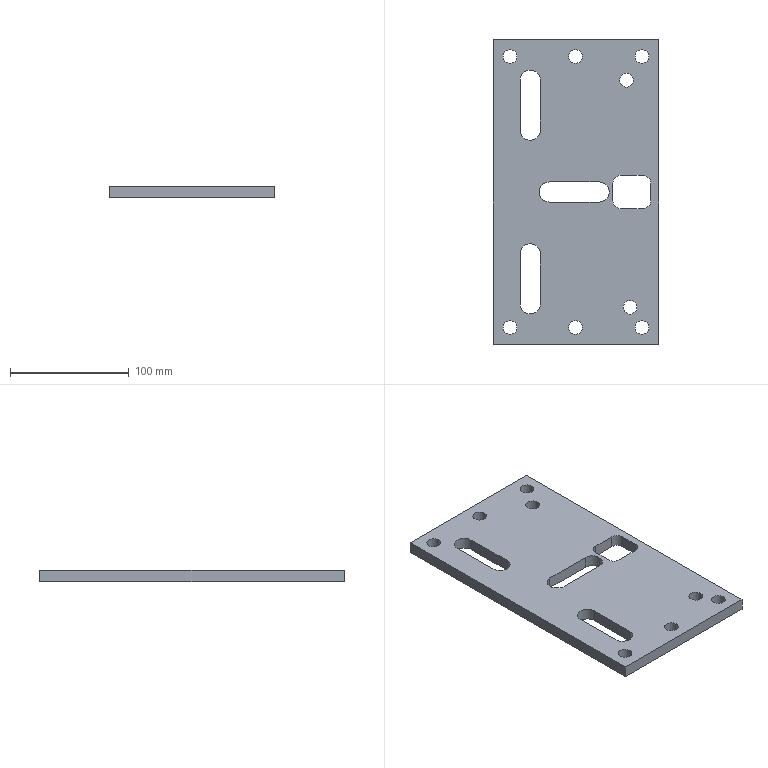Part | NX | features solid 2 | 1 solid | 34 faces | box 139 x 256 x 10 mm | volume 310704 mm3 | cylinder 18 | plane 16 | commonest cylinder face diameters 11.5 x8 17 x6 13 x4
STEP:
#1=CARTESIAN_POINT('',(344.5,-7.5,-36.5));
#2=VERTEX_POINT('',#1);
#3=CARTESIAN_POINT('',(338.,-14.,-36.5));
#4=VERTEX_POINT('',#3);
#5=CARTESIAN_POINT('',(338.,-7.5,-36.5));
#6=DIRECTION('',(0.,0.,-1.));
#7=DIRECTION('',(-1.,0.,0.));
#8=AXIS2_PLACEMENT_3D('',#5,#6,#7);
#9=CIRCLE('',#8,6.5);
#10=EDGE_CURVE('',#2,#4,#9,.T.);
#11=ORIENTED_EDGE('',*,*,#10,.T.);
#12=CARTESIAN_POINT('',(319.,-14.,-36.5));
#13=VERTEX_POINT('',#12);
#14=CARTESIAN_POINT('',(279.237,-14.,-36.5));
#15=DIRECTION('',(-1.,0.,0.));
#16=VECTOR('',#15,1000.);
#17=LINE('',#14,#16);
#18=EDGE_CURVE('',#4,#13,#17,.T.);
#19=ORIENTED_EDGE('',*,*,#18,.T.);
#20=CARTESIAN_POINT('',(312.5,-7.5,-36.5));
#21=VERTEX_POINT('',#20);
#22=CARTESIAN_POINT('',(319.,-7.5,-36.5));
#23=DIRECTION('',(0.,0.,-1.));
#24=DIRECTION('',(-1.,0.,0.));
#25=AXIS2_PLACEMENT_3D('',#22,#23,#24);
#26=CIRCLE('',#25,6.5);
#27=EDGE_CURVE('',#13,#21,#26,.T.);
#28=ORIENTED_EDGE('',*,*,#27,.T.);
#29=CARTESIAN_POINT('',(312.5,7.5,-36.5));
#30=VERTEX_POINT('',#29);
#31=CARTESIAN_POINT('',(312.5,0.,-36.5));
#32=DIRECTION('',(0.,1.,0.));
#33=VECTOR('',#32,1000.);
#34=LINE('',#31,#33);
#35=EDGE_CURVE('',#21,#30,#34,.T.);
#36=ORIENTED_EDGE('',*,*,#35,.T.);
#37=CARTESIAN_POINT('',(319.,14.,-36.5));
#38=VERTEX_POINT('',#37);
#39=CARTESIAN_POINT('',(319.,7.5,-36.5));
#40=DIRECTION('',(0.,0.,-1.));
#41=DIRECTION('',(-1.,0.,0.));
#42=AXIS2_PLACEMENT_3D('',#39,#40,#41);
#43=CIRCLE('',#42,6.5);
#44=EDGE_CURVE('',#30,#38,#43,.T.);
#45=ORIENTED_EDGE('',*,*,#44,.T.);
#46=CARTESIAN_POINT('',(338.,14.,-36.5));
#47=VERTEX_POINT('',#46);
#48=CARTESIAN_POINT('',(279.237,14.,-36.5));
#49=DIRECTION('',(1.,0.,0.));
#50=VECTOR('',#49,1000.);
#51=LINE('',#48,#50);
#52=EDGE_CURVE('',#38,#47,#51,.T.);
#53=ORIENTED_EDGE('',*,*,#52,.T.);
#54=CARTESIAN_POINT('',(344.5,7.5,-36.5));
#55=VERTEX_POINT('',#54);
#56=CARTESIAN_POINT('',(338.,7.5,-36.5));
#57=DIRECTION('',(0.,0.,-1.));
#58=DIRECTION('',(-1.,0.,0.));
#59=AXIS2_PLACEMENT_3D('',#56,#57,#58);
#60=CIRCLE('',#59,6.5);
#61=EDGE_CURVE('',#47,#55,#60,.T.);
#62=ORIENTED_EDGE('',*,*,#61,.T.);
#63=CARTESIAN_POINT('',(344.5,0.,-36.5));
#64=DIRECTION('',(0.,-1.,0.));
#65=VECTOR('',#64,1000.);
#66=LINE('',#63,#65);
#67=EDGE_CURVE('',#55,#2,#66,.T.);
#68=ORIENTED_EDGE('',*,*,#67,.T.);
#69=EDGE_LOOP('',(#11,#19,#28,#36,#45,#53,#62,#68));
#70=FACE_BOUND('',#69,.T.);
#71=CARTESIAN_POINT('',(259.,-8.5,-36.5));
#72=VERTEX_POINT('',#71);
#73=CARTESIAN_POINT('',(301.,-8.5,-36.5));
#74=VERTEX_POINT('',#73);
#75=CARTESIAN_POINT('',(259.,-8.5,-36.5));
#76=DIRECTION('',(1.,0.,0.));
#77=VECTOR('',#76,1000.);
#78=LINE('',#75,#77);
#79=EDGE_CURVE('',#72,#74,#78,.T.);
#80=ORIENTED_EDGE('',*,*,#79,.F.);
#81=CARTESIAN_POINT('',(259.,8.5,-36.5));
#82=VERTEX_POINT('',#81);
#83=CARTESIAN_POINT('',(259.,0.,-36.5));
#84=DIRECTION('',(0.,0.,-1.));
#85=DIRECTION('',(-1.,0.,0.));
#86=AXIS2_PLACEMENT_3D('',#83,#84,#85);
#87=CIRCLE('',#86,8.5);
#88=EDGE_CURVE('',#82,#72,#87,.F.);
#89=ORIENTED_EDGE('',*,*,#88,.F.);
#90=CARTESIAN_POINT('',(301.,8.5,-36.5));
#91=VERTEX_POINT('',#90);
#92=CARTESIAN_POINT('',(276.237,8.5,-36.5));
#93=DIRECTION('',(1.,0.,0.));
#94=VECTOR('',#93,1000.);
#95=LINE('',#92,#94);
#96=EDGE_CURVE('',#82,#91,#95,.T.);
#97=ORIENTED_EDGE('',*,*,#96,.T.);
#98=CARTESIAN_POINT('',(301.,0.,-36.5));
#99=DIRECTION('',(0.,0.,-1.));
#100=DIRECTION('',(-1.,0.,0.));
#101=AXIS2_PLACEMENT_3D('',#98,#99,#100);
#102=CIRCLE('',#101,8.5);
#103=EDGE_CURVE('',#91,#74,#102,.T.);
#104=ORIENTED_EDGE('',*,*,#103,.T.);
#105=EDGE_LOOP('',(#80,#89,#97,#104));
#106=FACE_BOUND('',#105,.T.);
#107=CARTESIAN_POINT('',(234.5,52.,-36.5));
#108=VERTEX_POINT('',#107);
#109=CARTESIAN_POINT('',(251.5,52.,-36.5));
#110=VERTEX_POINT('',#109);
#111=CARTESIAN_POINT('',(243.,52.,-36.5));
#112=DIRECTION('',(0.,0.,-1.));
#113=DIRECTION('',(-1.,0.,0.));
#114=AXIS2_PLACEMENT_3D('',#111,#112,#113);
#115=CIRCLE('',#114,8.5);
#116=EDGE_CURVE('',#108,#110,#115,.F.);
#117=ORIENTED_EDGE('',*,*,#116,.F.);
#118=CARTESIAN_POINT('',(234.5,94.,-36.5));
#119=VERTEX_POINT('',#118);
#120=CARTESIAN_POINT('',(234.5,94.,-36.5));
#121=DIRECTION('',(0.,-1.,0.));
#122=VECTOR('',#121,1000.);
#123=LINE('',#120,#122);
#124=EDGE_CURVE('',#119,#108,#123,.T.);
#125=ORIENTED_EDGE('',*,*,#124,.F.);
#126=CARTESIAN_POINT('',(251.5,94.,-36.5));
#127=VERTEX_POINT('',#126);
#128=CARTESIAN_POINT('',(243.,94.,-36.5));
#129=DIRECTION('',(0.,0.,-1.));
#130=DIRECTION('',(-1.,0.,0.));
#131=AXIS2_PLACEMENT_3D('',#128,#129,#130);
#132=CIRCLE('',#131,8.5);
#133=EDGE_CURVE('',#127,#119,#132,.F.);
#134=ORIENTED_EDGE('',*,*,#133,.F.);
#135=CARTESIAN_POINT('',(251.5,52.,-36.5));
#136=DIRECTION('',(0.,1.,0.));
#137=VECTOR('',#136,1000.);
#138=LINE('',#135,#137);
#139=EDGE_CURVE('',#110,#127,#138,.T.);
#140=ORIENTED_EDGE('',*,*,#139,.F.);
#141=EDGE_LOOP('',(#117,#125,#134,#140));
#142=FACE_BOUND('',#141,.T.);
#143=CARTESIAN_POINT('',(331.25,-114.,-36.5));
#144=VERTEX_POINT('',#143);
#145=CARTESIAN_POINT('',(337.,-114.,-36.5));
#146=DIRECTION('',(0.,0.,-1.));
#147=DIRECTION('',(-1.,0.,0.));
#148=AXIS2_PLACEMENT_3D('',#145,#146,#147);
#149=CIRCLE('',#148,5.75);
#150=EDGE_CURVE('',#144,#144,#149,.F.);
#151=ORIENTED_EDGE('',*,*,#150,.F.);
#152=EDGE_LOOP('',(#151));
#153=FACE_BOUND('',#152,.T.);
#154=CARTESIAN_POINT('',(275.25,-114.,-36.5));
#155=VERTEX_POINT('',#154);
#156=CARTESIAN_POINT('',(281.,-114.,-36.5));
#157=DIRECTION('',(0.,0.,-1.));
#158=DIRECTION('',(-1.,0.,0.));
#159=AXIS2_PLACEMENT_3D('',#156,#157,#158);
#160=CIRCLE('',#159,5.75);
#161=EDGE_CURVE('',#155,#155,#160,.F.);
#162=ORIENTED_EDGE('',*,*,#161,.F.);
#163=EDGE_LOOP('',(#162));
#164=FACE_BOUND('',#163,.T.);
#165=CARTESIAN_POINT('',(220.25,114.,-36.5));
#166=VERTEX_POINT('',#165);
#167=CARTESIAN_POINT('',(226.,114.,-36.5));
#168=DIRECTION('',(0.,0.,-1.));
#169=DIRECTION('',(-1.,0.,0.));
#170=AXIS2_PLACEMENT_3D('',#167,#168,#169);
#171=CIRCLE('',#170,5.75);
#172=EDGE_CURVE('',#166,#166,#171,.F.);
#173=ORIENTED_EDGE('',*,*,#172,.F.);
#174=EDGE_LOOP('',(#173));
#175=FACE_BOUND('',#174,.T.);
#176=CARTESIAN_POINT('',(321.25,-97.,-36.5));
#177=VERTEX_POINT('',#176);
#178=CARTESIAN_POINT('',(327.,-97.,-36.5));
#179=DIRECTION('',(0.,0.,-1.));
#180=DIRECTION('',(-1.,0.,0.));
#181=AXIS2_PLACEMENT_3D('',#178,#179,#180);
#182=CIRCLE('',#181,5.75);
#183=EDGE_CURVE('',#177,#177,#182,.T.);
#184=ORIENTED_EDGE('',*,*,#183,.T.);
#185=EDGE_LOOP('',(#184));
#186=FACE_BOUND('',#185,.T.);
#187=CARTESIAN_POINT('',(331.25,114.,-36.5));
#188=VERTEX_POINT('',#187);
#189=CARTESIAN_POINT('',(337.,114.,-36.5));
#190=DIRECTION('',(0.,0.,-1.));
#191=DIRECTION('',(-1.,0.,0.));
#192=AXIS2_PLACEMENT_3D('',#189,#190,#191);
#193=CIRCLE('',#192,5.75);
#194=EDGE_CURVE('',#188,#188,#193,.F.);
#195=ORIENTED_EDGE('',*,*,#194,.F.);
#196=EDGE_LOOP('',(#195));
#197=FACE_BOUND('',#196,.T.);
#198=CARTESIAN_POINT('',(351.,-128.,-36.5));
#199=VERTEX_POINT('',#198);
#200=CARTESIAN_POINT('',(351.,128.,-36.5));
#201=VERTEX_POINT('',#200);
#202=CARTESIAN_POINT('',(351.,108.,-36.5));
#203=DIRECTION('',(0.,1.,0.));
#204=VECTOR('',#203,1000.);
#205=LINE('',#202,#204);
#206=EDGE_CURVE('',#199,#201,#205,.T.);
#207=ORIENTED_EDGE('',*,*,#206,.T.);
#208=CARTESIAN_POINT('',(212.,128.,-36.5));
#209=VERTEX_POINT('',#208);
#210=CARTESIAN_POINT('',(279.237,128.,-36.5));
#211=DIRECTION('',(-1.,0.,0.));
#212=VECTOR('',#211,1000.);
#213=LINE('',#210,#212);
#214=EDGE_CURVE('',#201,#209,#213,.T.);
#215=ORIENTED_EDGE('',*,*,#214,.T.);
#216=CARTESIAN_POINT('',(212.,-128.,-36.5));
#217=VERTEX_POINT('',#216);
#218=CARTESIAN_POINT('',(212.,105.,-36.5));
#219=DIRECTION('',(0.,-1.,0.));
#220=VECTOR('',#219,1000.);
#221=LINE('',#218,#220);
#222=EDGE_CURVE('',#209,#217,#221,.T.);
#223=ORIENTED_EDGE('',*,*,#222,.T.);
#224=CARTESIAN_POINT('',(279.237,-128.,-36.5));
#225=DIRECTION('',(1.,0.,0.));
#226=VECTOR('',#225,1000.);
#227=LINE('',#224,#226);
#228=EDGE_CURVE('',#217,#199,#227,.T.);
#229=ORIENTED_EDGE('',*,*,#228,.T.);
#230=EDGE_LOOP('',(#207,#215,#223,#229));
#231=FACE_BOUND('',#230,.T.);
#232=CARTESIAN_POINT('',(275.25,114.,-36.5));
#233=VERTEX_POINT('',#232);
#234=CARTESIAN_POINT('',(281.,114.,-36.5));
#235=DIRECTION('',(0.,0.,-1.));
#236=DIRECTION('',(-1.,0.,0.));
#237=AXIS2_PLACEMENT_3D('',#234,#235,#236);
#238=CIRCLE('',#237,5.75);
#239=EDGE_CURVE('',#233,#233,#238,.F.);
#240=ORIENTED_EDGE('',*,*,#239,.F.);
#241=EDGE_LOOP('',(#240));
#242=FACE_BOUND('',#241,.T.);
#243=CARTESIAN_POINT('',(220.25,-114.,-36.5));
#244=VERTEX_POINT('',#243);
#245=CARTESIAN_POINT('',(226.,-114.,-36.5));
#246=DIRECTION('',(0.,0.,-1.));
#247=DIRECTION('',(-1.,0.,0.));
#248=AXIS2_PLACEMENT_3D('',#245,#246,#247);
#249=CIRCLE('',#248,5.75);
#250=EDGE_CURVE('',#244,#244,#249,.F.);
#251=ORIENTED_EDGE('',*,*,#250,.F.);
#252=EDGE_LOOP('',(#251));
#253=FACE_BOUND('',#252,.T.);
#254=CARTESIAN_POINT('',(318.25,94.,-36.5));
#255=VERTEX_POINT('',#254);
#256=CARTESIAN_POINT('',(324.,94.,-36.5));
#257=DIRECTION('',(0.,0.,-1.));
#258=DIRECTION('',(-1.,0.,0.));
#259=AXIS2_PLACEMENT_3D('',#256,#257,#258);
#260=CIRCLE('',#259,5.75);
#261=EDGE_CURVE('',#255,#255,#260,.F.);
#262=ORIENTED_EDGE('',*,*,#261,.F.);
#263=EDGE_LOOP('',(#262));
#264=FACE_BOUND('',#263,.T.);
#265=CARTESIAN_POINT('',(234.5,-52.,-36.5));
#266=VERTEX_POINT('',#265);
#267=CARTESIAN_POINT('',(234.5,-94.,-36.5));
#268=VERTEX_POINT('',#267);
#269=CARTESIAN_POINT('',(234.5,0.,-36.5));
#270=DIRECTION('',(0.,-1.,0.));
#271=VECTOR('',#270,1000.);
#272=LINE('',#269,#271);
#273=EDGE_CURVE('',#266,#268,#272,.T.);
#274=ORIENTED_EDGE('',*,*,#273,.F.);
#275=CARTESIAN_POINT('',(251.5,-52.,-36.5));
#276=VERTEX_POINT('',#275);
#277=CARTESIAN_POINT('',(243.,-52.,-36.5));
#278=DIRECTION('',(0.,0.,-1.));
#279=DIRECTION('',(-1.,0.,0.));
#280=AXIS2_PLACEMENT_3D('',#277,#278,#279);
#281=CIRCLE('',#280,8.5);
#282=EDGE_CURVE('',#276,#266,#281,.F.);
#283=ORIENTED_EDGE('',*,*,#282,.F.);
#284=CARTESIAN_POINT('',(251.5,-94.,-36.5));
#285=VERTEX_POINT('',#284);
#286=CARTESIAN_POINT('',(251.5,0.,-36.5));
#287=DIRECTION('',(0.,1.,0.));
#288=VECTOR('',#287,1000.);
#289=LINE('',#286,#288);
#290=EDGE_CURVE('',#285,#276,#289,.T.);
#291=ORIENTED_EDGE('',*,*,#290,.F.);
#292=CARTESIAN_POINT('',(243.,-94.,-36.5));
#293=DIRECTION('',(0.,0.,-1.));
#294=DIRECTION('',(-1.,0.,0.));
#295=AXIS2_PLACEMENT_3D('',#292,#293,#294);
#296=CIRCLE('',#295,8.5);
#297=EDGE_CURVE('',#285,#268,#296,.T.);
#298=ORIENTED_EDGE('',*,*,#297,.T.);
#299=EDGE_LOOP('',(#274,#283,#291,#298));
#300=FACE_BOUND('',#299,.T.);
#301=CARTESIAN_POINT('',(279.237,0.,-36.5));
#302=DIRECTION('',(0.,0.,-1.));
#303=DIRECTION('',(-1.,0.,0.));
#304=AXIS2_PLACEMENT_3D('',#301,#302,#303);
#305=PLANE('',#304);
#306=ADVANCED_FACE('',(#70,#106,#142,#153,#164,#175,#186,#197,#231,#242,#253,#264,#300),#305,.F.);
#307=CARTESIAN_POINT('',(338.,-14.,-46.5));
#308=VERTEX_POINT('',#307);
#309=CARTESIAN_POINT('',(319.,-14.,-46.5));
#310=VERTEX_POINT('',#309);
#311=CARTESIAN_POINT('',(279.237,-14.,-46.5));
#312=DIRECTION('',(-1.,0.,0.));
#313=VECTOR('',#312,1000.);
#314=LINE('',#311,#313);
#315=EDGE_CURVE('',#308,#310,#314,.T.);
#316=ORIENTED_EDGE('',*,*,#315,.F.);
#317=CARTESIAN_POINT('',(344.5,-7.5,-46.5));
#318=VERTEX_POINT('',#317);
#319=CARTESIAN_POINT('',(338.,-7.5,-46.5));
#320=DIRECTION('',(0.,0.,-1.));
#321=DIRECTION('',(-1.,0.,0.));
#322=AXIS2_PLACEMENT_3D('',#319,#320,#321);
#323=CIRCLE('',#322,6.5);
#324=EDGE_CURVE('',#318,#308,#323,.T.);
#325=ORIENTED_EDGE('',*,*,#324,.F.);
#326=CARTESIAN_POINT('',(344.5,7.5,-46.5));
#327=VERTEX_POINT('',#326);
#328=CARTESIAN_POINT('',(344.5,0.,-46.5));
#329=DIRECTION('',(0.,-1.,0.));
#330=VECTOR('',#329,1000.);
#331=LINE('',#328,#330);
#332=EDGE_CURVE('',#327,#318,#331,.T.);
#333=ORIENTED_EDGE('',*,*,#332,.F.);
#334=CARTESIAN_POINT('',(338.,14.,-46.5));
#335=VERTEX_POINT('',#334);
#336=CARTESIAN_POINT('',(338.,7.5,-46.5));
#337=DIRECTION('',(0.,0.,-1.));
#338=DIRECTION('',(-1.,0.,0.));
#339=AXIS2_PLACEMENT_3D('',#336,#337,#338);
#340=CIRCLE('',#339,6.5);
#341=EDGE_CURVE('',#335,#327,#340,.T.);
#342=ORIENTED_EDGE('',*,*,#341,.F.);
#343=CARTESIAN_POINT('',(319.,14.,-46.5));
#344=VERTEX_POINT('',#343);
#345=CARTESIAN_POINT('',(279.237,14.,-46.5));
#346=DIRECTION('',(1.,0.,0.));
#347=VECTOR('',#346,1000.);
#348=LINE('',#345,#347);
#349=EDGE_CURVE('',#344,#335,#348,.T.);
#350=ORIENTED_EDGE('',*,*,#349,.F.);
#351=CARTESIAN_POINT('',(312.5,7.5,-46.5));
#352=VERTEX_POINT('',#351);
#353=CARTESIAN_POINT('',(319.,7.5,-46.5));
#354=DIRECTION('',(0.,0.,-1.));
#355=DIRECTION('',(-1.,0.,0.));
#356=AXIS2_PLACEMENT_3D('',#353,#354,#355);
#357=CIRCLE('',#356,6.5);
#358=EDGE_CURVE('',#352,#344,#357,.T.);
#359=ORIENTED_EDGE('',*,*,#358,.F.);
#360=CARTESIAN_POINT('',(312.5,-7.5,-46.5));
#361=VERTEX_POINT('',#360);
#362=CARTESIAN_POINT('',(312.5,0.,-46.5));
#363=DIRECTION('',(0.,1.,0.));
#364=VECTOR('',#363,1000.);
#365=LINE('',#362,#364);
#366=EDGE_CURVE('',#361,#352,#365,.T.);
#367=ORIENTED_EDGE('',*,*,#366,.F.);
#368=CARTESIAN_POINT('',(319.,-7.5,-46.5));
#369=DIRECTION('',(0.,0.,-1.));
#370=DIRECTION('',(-1.,0.,0.));
#371=AXIS2_PLACEMENT_3D('',#368,#369,#370);
#372=CIRCLE('',#371,6.5);
#373=EDGE_CURVE('',#310,#361,#372,.T.);
#374=ORIENTED_EDGE('',*,*,#373,.F.);
#375=EDGE_LOOP('',(#316,#325,#333,#342,#350,#359,#367,#374));
#376=FACE_BOUND('',#375,.T.);
#377=CARTESIAN_POINT('',(259.,-8.5,-46.5));
#378=VERTEX_POINT('',#377);
#379=CARTESIAN_POINT('',(259.,8.5,-46.5));
#380=VERTEX_POINT('',#379);
#381=CARTESIAN_POINT('',(259.,0.,-46.5));
#382=DIRECTION('',(0.,0.,-1.));
#383=DIRECTION('',(-1.,0.,0.));
#384=AXIS2_PLACEMENT_3D('',#381,#382,#383);
#385=CIRCLE('',#384,8.5);
#386=EDGE_CURVE('',#378,#380,#385,.T.);
#387=ORIENTED_EDGE('',*,*,#386,.F.);
#388=CARTESIAN_POINT('',(301.,-8.5,-46.5));
#389=VERTEX_POINT('',#388);
#390=CARTESIAN_POINT('',(259.,-8.5,-46.5));
#391=DIRECTION('',(1.,0.,0.));
#392=VECTOR('',#391,1000.);
#393=LINE('',#390,#392);
#394=EDGE_CURVE('',#378,#389,#393,.T.);
#395=ORIENTED_EDGE('',*,*,#394,.T.);
#396=CARTESIAN_POINT('',(301.,8.5,-46.5));
#397=VERTEX_POINT('',#396);
#398=CARTESIAN_POINT('',(301.,0.,-46.5));
#399=DIRECTION('',(0.,0.,-1.));
#400=DIRECTION('',(-1.,0.,0.));
#401=AXIS2_PLACEMENT_3D('',#398,#399,#400);
#402=CIRCLE('',#401,8.5);
#403=EDGE_CURVE('',#397,#389,#402,.T.);
#404=ORIENTED_EDGE('',*,*,#403,.F.);
#405=CARTESIAN_POINT('',(301.,8.5,-46.5));
#406=DIRECTION('',(-1.,0.,0.));
#407=VECTOR('',#406,1000.);
#408=LINE('',#405,#407);
#409=EDGE_CURVE('',#397,#380,#408,.T.);
#410=ORIENTED_EDGE('',*,*,#409,.T.);
#411=EDGE_LOOP('',(#387,#395,#404,#410));
#412=FACE_BOUND('',#411,.T.);
#413=CARTESIAN_POINT('',(234.5,94.,-46.5));
#414=VERTEX_POINT('',#413);
#415=CARTESIAN_POINT('',(234.5,52.,-46.5));
#416=VERTEX_POINT('',#415);
#417=CARTESIAN_POINT('',(234.5,94.,-46.5));
#418=DIRECTION('',(0.,-1.,0.));
#419=VECTOR('',#418,1000.);
#420=LINE('',#417,#419);
#421=EDGE_CURVE('',#414,#416,#420,.T.);
#422=ORIENTED_EDGE('',*,*,#421,.T.);
#423=CARTESIAN_POINT('',(251.5,52.,-46.5));
#424=VERTEX_POINT('',#423);
#425=CARTESIAN_POINT('',(243.,52.,-46.5));
#426=DIRECTION('',(0.,0.,-1.));
#427=DIRECTION('',(-1.,0.,0.));
#428=AXIS2_PLACEMENT_3D('',#425,#426,#427);
#429=CIRCLE('',#428,8.5);
#430=EDGE_CURVE('',#424,#416,#429,.T.);
#431=ORIENTED_EDGE('',*,*,#430,.F.);
#432=CARTESIAN_POINT('',(251.5,94.,-46.5));
#433=VERTEX_POINT('',#432);
#434=CARTESIAN_POINT('',(251.5,52.,-46.5));
#435=DIRECTION('',(0.,1.,0.));
#436=VECTOR('',#435,1000.);
#437=LINE('',#434,#436);
#438=EDGE_CURVE('',#424,#433,#437,.T.);
#439=ORIENTED_EDGE('',*,*,#438,.T.);
#440=CARTESIAN_POINT('',(243.,94.,-46.5));
#441=DIRECTION('',(0.,0.,-1.));
#442=DIRECTION('',(-1.,0.,0.));
#443=AXIS2_PLACEMENT_3D('',#440,#441,#442);
#444=CIRCLE('',#443,8.5);
#445=EDGE_CURVE('',#433,#414,#444,.F.);
#446=ORIENTED_EDGE('',*,*,#445,.T.);
#447=EDGE_LOOP('',(#422,#431,#439,#446));
#448=FACE_BOUND('',#447,.T.);
#449=CARTESIAN_POINT('',(331.25,-114.,-46.5));
#450=VERTEX_POINT('',#449);
#451=CARTESIAN_POINT('',(337.,-114.,-46.5));
#452=DIRECTION('',(0.,0.,-1.));
#453=DIRECTION('',(-1.,0.,0.));
#454=AXIS2_PLACEMENT_3D('',#451,#452,#453);
#455=CIRCLE('',#454,5.75);
#456=EDGE_CURVE('',#450,#450,#455,.F.);
#457=ORIENTED_EDGE('',*,*,#456,.T.);
#458=EDGE_LOOP('',(#457));
#459=FACE_BOUND('',#458,.T.);
#460=CARTESIAN_POINT('',(275.25,-114.,-46.5));
#461=VERTEX_POINT('',#460);
#462=CARTESIAN_POINT('',(281.,-114.,-46.5));
#463=DIRECTION('',(0.,0.,-1.));
#464=DIRECTION('',(-1.,0.,0.));
#465=AXIS2_PLACEMENT_3D('',#462,#463,#464);
#466=CIRCLE('',#465,5.75);
#467=EDGE_CURVE('',#461,#461,#466,.F.);
#468=ORIENTED_EDGE('',*,*,#467,.T.);
#469=EDGE_LOOP('',(#468));
#470=FACE_BOUND('',#469,.T.);
#471=CARTESIAN_POINT('',(220.25,114.,-46.5));
#472=VERTEX_POINT('',#471);
#473=CARTESIAN_POINT('',(226.,114.,-46.5));
#474=DIRECTION('',(0.,0.,-1.));
#475=DIRECTION('',(-1.,0.,0.));
#476=AXIS2_PLACEMENT_3D('',#473,#474,#475);
#477=CIRCLE('',#476,5.75);
#478=EDGE_CURVE('',#472,#472,#477,.F.);
#479=ORIENTED_EDGE('',*,*,#478,.T.);
#480=EDGE_LOOP('',(#479));
#481=FACE_BOUND('',#480,.T.);
#482=CARTESIAN_POINT('',(321.25,-97.,-46.5));
#483=VERTEX_POINT('',#482);
#484=CARTESIAN_POINT('',(327.,-97.,-46.5));
#485=DIRECTION('',(0.,0.,-1.));
#486=DIRECTION('',(-1.,0.,0.));
#487=AXIS2_PLACEMENT_3D('',#484,#485,#486);
#488=CIRCLE('',#487,5.75);
#489=EDGE_CURVE('',#483,#483,#488,.F.);
#490=ORIENTED_EDGE('',*,*,#489,.T.);
#491=EDGE_LOOP('',(#490));
#492=FACE_BOUND('',#491,.T.);
#493=CARTESIAN_POINT('',(331.25,114.,-46.5));
#494=VERTEX_POINT('',#493);
#495=CARTESIAN_POINT('',(337.,114.,-46.5));
#496=DIRECTION('',(0.,0.,-1.));
#497=DIRECTION('',(-1.,0.,0.));
#498=AXIS2_PLACEMENT_3D('',#495,#496,#497);
#499=CIRCLE('',#498,5.75);
#500=EDGE_CURVE('',#494,#494,#499,.F.);
#501=ORIENTED_EDGE('',*,*,#500,.T.);
#502=EDGE_LOOP('',(#501));
#503=FACE_BOUND('',#502,.T.);
#504=CARTESIAN_POINT('',(351.,-128.,-46.5));
#505=VERTEX_POINT('',#504);
#506=CARTESIAN_POINT('',(351.,128.,-46.5));
#507=VERTEX_POINT('',#506);
#508=CARTESIAN_POINT('',(351.,108.,-46.5));
#509=DIRECTION('',(0.,1.,0.));
#510=VECTOR('',#509,1000.);
#511=LINE('',#508,#510);
#512=EDGE_CURVE('',#505,#507,#511,.T.);
#513=ORIENTED_EDGE('',*,*,#512,.F.);
#514=CARTESIAN_POINT('',(212.,-128.,-46.5));
#515=VERTEX_POINT('',#514);
#516=CARTESIAN_POINT('',(279.237,-128.,-46.5));
#517=DIRECTION('',(1.,0.,0.));
#518=VECTOR('',#517,1000.);
#519=LINE('',#516,#518);
#520=EDGE_CURVE('',#515,#505,#519,.T.);
#521=ORIENTED_EDGE('',*,*,#520,.F.);
#522=CARTESIAN_POINT('',(212.,128.,-46.5));
#523=VERTEX_POINT('',#522);
#524=CARTESIAN_POINT('',(212.,105.,-46.5));
#525=DIRECTION('',(0.,-1.,0.));
#526=VECTOR('',#525,1000.);
#527=LINE('',#524,#526);
#528=EDGE_CURVE('',#523,#515,#527,.T.);
#529=ORIENTED_EDGE('',*,*,#528,.F.);
#530=CARTESIAN_POINT('',(279.237,128.,-46.5));
#531=DIRECTION('',(-1.,0.,0.));
#532=VECTOR('',#531,1000.);
#533=LINE('',#530,#532);
#534=EDGE_CURVE('',#507,#523,#533,.T.);
#535=ORIENTED_EDGE('',*,*,#534,.F.);
#536=EDGE_LOOP('',(#513,#521,#529,#535));
#537=FACE_BOUND('',#536,.T.);
#538=CARTESIAN_POINT('',(275.25,114.,-46.5));
#539=VERTEX_POINT('',#538);
#540=CARTESIAN_POINT('',(281.,114.,-46.5));
#541=DIRECTION('',(0.,0.,-1.));
#542=DIRECTION('',(-1.,0.,0.));
#543=AXIS2_PLACEMENT_3D('',#540,#541,#542);
#544=CIRCLE('',#543,5.75);
#545=EDGE_CURVE('',#539,#539,#544,.T.);
#546=ORIENTED_EDGE('',*,*,#545,.F.);
#547=EDGE_LOOP('',(#546));
#548=FACE_BOUND('',#547,.T.);
#549=CARTESIAN_POINT('',(220.25,-114.,-46.5));
#550=VERTEX_POINT('',#549);
#551=CARTESIAN_POINT('',(226.,-114.,-46.5));
#552=DIRECTION('',(0.,0.,-1.));
#553=DIRECTION('',(-1.,0.,0.));
#554=AXIS2_PLACEMENT_3D('',#551,#552,#553);
#555=CIRCLE('',#554,5.75);
#556=EDGE_CURVE('',#550,#550,#555,.F.);
#557=ORIENTED_EDGE('',*,*,#556,.T.);
#558=EDGE_LOOP('',(#557));
#559=FACE_BOUND('',#558,.T.);
#560=CARTESIAN_POINT('',(318.25,94.,-46.5));
#561=VERTEX_POINT('',#560);
#562=CARTESIAN_POINT('',(324.,94.,-46.5));
#563=DIRECTION('',(0.,0.,-1.));
#564=DIRECTION('',(-1.,0.,0.));
#565=AXIS2_PLACEMENT_3D('',#562,#563,#564);
#566=CIRCLE('',#565,5.75);
#567=EDGE_CURVE('',#561,#561,#566,.T.);
#568=ORIENTED_EDGE('',*,*,#567,.F.);
#569=EDGE_LOOP('',(#568));
#570=FACE_BOUND('',#569,.T.);
#571=CARTESIAN_POINT('',(251.5,-52.,-46.5));
#572=VERTEX_POINT('',#571);
#573=CARTESIAN_POINT('',(234.5,-52.,-46.5));
#574=VERTEX_POINT('',#573);
#575=CARTESIAN_POINT('',(243.,-52.,-46.5));
#576=DIRECTION('',(0.,0.,-1.));
#577=DIRECTION('',(-1.,0.,0.));
#578=AXIS2_PLACEMENT_3D('',#575,#576,#577);
#579=CIRCLE('',#578,8.5);
#580=EDGE_CURVE('',#572,#574,#579,.F.);
#581=ORIENTED_EDGE('',*,*,#580,.T.);
#582=CARTESIAN_POINT('',(234.5,-94.,-46.5));
#583=VERTEX_POINT('',#582);
#584=CARTESIAN_POINT('',(234.5,-94.,-46.5));
#585=DIRECTION('',(0.,1.,0.));
#586=VECTOR('',#585,1000.);
#587=LINE('',#584,#586);
#588=EDGE_CURVE('',#583,#574,#587,.T.);
#589=ORIENTED_EDGE('',*,*,#588,.F.);
#590=CARTESIAN_POINT('',(251.5,-94.,-46.5));
#591=VERTEX_POINT('',#590);
#592=CARTESIAN_POINT('',(243.,-94.,-46.5));
#593=DIRECTION('',(0.,0.,-1.));
#594=DIRECTION('',(-1.,0.,0.));
#595=AXIS2_PLACEMENT_3D('',#592,#593,#594);
#596=CIRCLE('',#595,8.5);
#597=EDGE_CURVE('',#591,#583,#596,.T.);
#598=ORIENTED_EDGE('',*,*,#597,.F.);
#599=CARTESIAN_POINT('',(251.5,0.,-46.5));
#600=DIRECTION('',(0.,1.,0.));
#601=VECTOR('',#600,1000.);
#602=LINE('',#599,#601);
#603=EDGE_CURVE('',#591,#572,#602,.T.);
#604=ORIENTED_EDGE('',*,*,#603,.T.);
#605=EDGE_LOOP('',(#581,#589,#598,#604));
#606=FACE_BOUND('',#605,.T.);
#607=CARTESIAN_POINT('',(279.237,0.,-46.5));
#608=DIRECTION('',(0.,0.,-1.));
#609=DIRECTION('',(-1.,0.,0.));
#610=AXIS2_PLACEMENT_3D('',#607,#608,#609);
#611=PLANE('',#610);
#612=ADVANCED_FACE('',(#376,#412,#448,#459,#470,#481,#492,#503,#537,#548,#559,#570,#606),#611,.T.);
#613=ORIENTED_EDGE('',*,*,#206,.F.);
#614=CARTESIAN_POINT('',(351.,-128.,-6.49));
#615=DIRECTION('',(0.,0.,1.));
#616=VECTOR('',#615,1000.);
#617=LINE('',#614,#616);
#618=EDGE_CURVE('',#505,#199,#617,.T.);
#619=ORIENTED_EDGE('',*,*,#618,.F.);
#620=ORIENTED_EDGE('',*,*,#512,.T.);
#621=CARTESIAN_POINT('',(351.,128.,-46.5));
#622=DIRECTION('',(0.,0.,1.));
#623=VECTOR('',#622,1000.);
#624=LINE('',#621,#623);
#625=EDGE_CURVE('',#507,#201,#624,.T.);
#626=ORIENTED_EDGE('',*,*,#625,.T.);
#627=EDGE_LOOP('',(#613,#619,#620,#626));
#628=FACE_BOUND('',#627,.T.);
#629=CARTESIAN_POINT('',(351.,108.,-46.5));
#630=DIRECTION('',(1.,0.,0.));
#631=DIRECTION('',(0.,0.,-1.));
#632=AXIS2_PLACEMENT_3D('',#629,#630,#631);
#633=PLANE('',#632);
#634=ADVANCED_FACE('',(#628),#633,.T.);
#635=ORIENTED_EDGE('',*,*,#228,.F.);
#636=CARTESIAN_POINT('',(212.,-128.,-46.5));
#637=DIRECTION('',(0.,0.,1.));
#638=VECTOR('',#637,1000.);
#639=LINE('',#636,#638);
#640=EDGE_CURVE('',#515,#217,#639,.T.);
#641=ORIENTED_EDGE('',*,*,#640,.F.);
#642=ORIENTED_EDGE('',*,*,#520,.T.);
#643=ORIENTED_EDGE('',*,*,#618,.T.);
#644=EDGE_LOOP('',(#635,#641,#642,#643));
#645=FACE_BOUND('',#644,.T.);
#646=CARTESIAN_POINT('',(279.237,-128.,-6.49));
#647=DIRECTION('',(0.,-1.,0.));
#648=DIRECTION('',(0.,0.,-1.));
#649=AXIS2_PLACEMENT_3D('',#646,#647,#648);
#650=PLANE('',#649);
#651=ADVANCED_FACE('',(#645),#650,.T.);
#652=ORIENTED_EDGE('',*,*,#222,.F.);
#653=CARTESIAN_POINT('',(212.,128.,-6.49));
#654=DIRECTION('',(0.,0.,1.));
#655=VECTOR('',#654,1000.);
#656=LINE('',#653,#655);
#657=EDGE_CURVE('',#523,#209,#656,.T.);
#658=ORIENTED_EDGE('',*,*,#657,.F.);
#659=ORIENTED_EDGE('',*,*,#528,.T.);
#660=ORIENTED_EDGE('',*,*,#640,.T.);
#661=EDGE_LOOP('',(#652,#658,#659,#660));
#662=FACE_BOUND('',#661,.T.);
#663=CARTESIAN_POINT('',(212.,105.,-46.5));
#664=DIRECTION('',(-1.,0.,0.));
#665=DIRECTION('',(0.,0.,1.));
#666=AXIS2_PLACEMENT_3D('',#663,#664,#665);
#667=PLANE('',#666);
#668=ADVANCED_FACE('',(#662),#667,.T.);
#669=ORIENTED_EDGE('',*,*,#214,.F.);
#670=ORIENTED_EDGE('',*,*,#625,.F.);
#671=ORIENTED_EDGE('',*,*,#534,.T.);
#672=ORIENTED_EDGE('',*,*,#657,.T.);
#673=EDGE_LOOP('',(#669,#670,#671,#672));
#674=FACE_BOUND('',#673,.T.);
#675=CARTESIAN_POINT('',(279.237,128.,-6.49));
#676=DIRECTION('',(0.,1.,0.));
#677=DIRECTION('',(0.,0.,1.));
#678=AXIS2_PLACEMENT_3D('',#675,#676,#677);
#679=PLANE('',#678);
#680=ADVANCED_FACE('',(#674),#679,.T.);
#681=ORIENTED_EDGE('',*,*,#500,.F.);
#682=EDGE_LOOP('',(#681));
#683=FACE_BOUND('',#682,.T.);
#684=ORIENTED_EDGE('',*,*,#194,.T.);
#685=EDGE_LOOP('',(#684));
#686=FACE_BOUND('',#685,.T.);
#687=CARTESIAN_POINT('',(337.,114.,-109.5));
#688=DIRECTION('',(0.,0.,1.));
#689=DIRECTION('',(1.,0.,0.));
#690=AXIS2_PLACEMENT_3D('',#687,#688,#689);
#691=CYLINDRICAL_SURFACE('',#690,5.75);
#692=ADVANCED_FACE('',(#683,#686),#691,.F.);
#693=ORIENTED_EDGE('',*,*,#489,.F.);
#694=EDGE_LOOP('',(#693));
#695=FACE_BOUND('',#694,.T.);
#696=ORIENTED_EDGE('',*,*,#183,.F.);
#697=EDGE_LOOP('',(#696));
#698=FACE_BOUND('',#697,.T.);
#699=CARTESIAN_POINT('',(327.,-97.,-109.5));
#700=DIRECTION('',(0.,0.,1.));
#701=DIRECTION('',(1.,0.,0.));
#702=AXIS2_PLACEMENT_3D('',#699,#700,#701);
#703=CYLINDRICAL_SURFACE('',#702,5.75);
#704=ADVANCED_FACE('',(#695,#698),#703,.F.);
#705=ORIENTED_EDGE('',*,*,#545,.T.);
#706=EDGE_LOOP('',(#705));
#707=FACE_BOUND('',#706,.T.);
#708=ORIENTED_EDGE('',*,*,#239,.T.);
#709=EDGE_LOOP('',(#708));
#710=FACE_BOUND('',#709,.T.);
#711=CARTESIAN_POINT('',(281.,114.,-109.5));
#712=DIRECTION('',(0.,0.,1.));
#713=DIRECTION('',(1.,0.,0.));
#714=AXIS2_PLACEMENT_3D('',#711,#712,#713);
#715=CYLINDRICAL_SURFACE('',#714,5.75);
#716=ADVANCED_FACE('',(#707,#710),#715,.F.);
#717=ORIENTED_EDGE('',*,*,#478,.F.);
#718=EDGE_LOOP('',(#717));
#719=FACE_BOUND('',#718,.T.);
#720=ORIENTED_EDGE('',*,*,#172,.T.);
#721=EDGE_LOOP('',(#720));
#722=FACE_BOUND('',#721,.T.);
#723=CARTESIAN_POINT('',(226.,114.,-109.5));
#724=DIRECTION('',(0.,0.,1.));
#725=DIRECTION('',(1.,0.,0.));
#726=AXIS2_PLACEMENT_3D('',#723,#724,#725);
#727=CYLINDRICAL_SURFACE('',#726,5.75);
#728=ADVANCED_FACE('',(#719,#722),#727,.F.);
#729=ORIENTED_EDGE('',*,*,#556,.F.);
#730=EDGE_LOOP('',(#729));
#731=FACE_BOUND('',#730,.T.);
#732=ORIENTED_EDGE('',*,*,#250,.T.);
#733=EDGE_LOOP('',(#732));
#734=FACE_BOUND('',#733,.T.);
#735=CARTESIAN_POINT('',(226.,-114.,-109.5));
#736=DIRECTION('',(0.,0.,1.));
#737=DIRECTION('',(1.,0.,0.));
#738=AXIS2_PLACEMENT_3D('',#735,#736,#737);
#739=CYLINDRICAL_SURFACE('',#738,5.75);
#740=ADVANCED_FACE('',(#731,#734),#739,.F.);
#741=ORIENTED_EDGE('',*,*,#467,.F.);
#742=EDGE_LOOP('',(#741));
#743=FACE_BOUND('',#742,.T.);
#744=ORIENTED_EDGE('',*,*,#161,.T.);
#745=EDGE_LOOP('',(#744));
#746=FACE_BOUND('',#745,.T.);
#747=CARTESIAN_POINT('',(281.,-114.,-109.5));
#748=DIRECTION('',(0.,0.,1.));
#749=DIRECTION('',(1.,0.,0.));
#750=AXIS2_PLACEMENT_3D('',#747,#748,#749);
#751=CYLINDRICAL_SURFACE('',#750,5.75);
#752=ADVANCED_FACE('',(#743,#746),#751,.F.);
#753=ORIENTED_EDGE('',*,*,#567,.T.);
#754=EDGE_LOOP('',(#753));
#755=FACE_BOUND('',#754,.T.);
#756=ORIENTED_EDGE('',*,*,#261,.T.);
#757=EDGE_LOOP('',(#756));
#758=FACE_BOUND('',#757,.T.);
#759=CARTESIAN_POINT('',(324.,94.,-109.5));
#760=DIRECTION('',(0.,0.,1.));
#761=DIRECTION('',(1.,0.,0.));
#762=AXIS2_PLACEMENT_3D('',#759,#760,#761);
#763=CYLINDRICAL_SURFACE('',#762,5.75);
#764=ADVANCED_FACE('',(#755,#758),#763,.F.);
#765=ORIENTED_EDGE('',*,*,#456,.F.);
#766=EDGE_LOOP('',(#765));
#767=FACE_BOUND('',#766,.T.);
#768=ORIENTED_EDGE('',*,*,#150,.T.);
#769=EDGE_LOOP('',(#768));
#770=FACE_BOUND('',#769,.T.);
#771=CARTESIAN_POINT('',(337.,-114.,-109.5));
#772=DIRECTION('',(0.,0.,1.));
#773=DIRECTION('',(1.,0.,0.));
#774=AXIS2_PLACEMENT_3D('',#771,#772,#773);
#775=CYLINDRICAL_SURFACE('',#774,5.75);
#776=ADVANCED_FACE('',(#767,#770),#775,.F.);
#777=CARTESIAN_POINT('',(234.5,-52.,-109.5));
#778=DIRECTION('',(0.,0.,-1.));
#779=VECTOR('',#778,1000.);
#780=LINE('',#777,#779);
#781=EDGE_CURVE('',#574,#266,#780,.F.);
#782=ORIENTED_EDGE('',*,*,#781,.T.);
#783=ORIENTED_EDGE('',*,*,#273,.T.);
#784=CARTESIAN_POINT('',(234.5,-94.,-109.5));
#785=DIRECTION('',(0.,0.,1.));
#786=VECTOR('',#785,1000.);
#787=LINE('',#784,#786);
#788=EDGE_CURVE('',#583,#268,#787,.T.);
#789=ORIENTED_EDGE('',*,*,#788,.F.);
#790=ORIENTED_EDGE('',*,*,#588,.T.);
#791=EDGE_LOOP('',(#782,#783,#789,#790));
#792=FACE_BOUND('',#791,.T.);
#793=CARTESIAN_POINT('',(234.5,-94.,-109.5));
#794=DIRECTION('',(1.,0.,0.));
#795=DIRECTION('',(0.,0.,-1.));
#796=AXIS2_PLACEMENT_3D('',#793,#794,#795);
#797=PLANE('',#796);
#798=ADVANCED_FACE('',(#792),#797,.T.);
#799=CARTESIAN_POINT('',(251.5,-52.,-109.5));
#800=DIRECTION('',(0.,0.,1.));
#801=VECTOR('',#800,1000.);
#802=LINE('',#799,#801);
#803=EDGE_CURVE('',#572,#276,#802,.T.);
#804=ORIENTED_EDGE('',*,*,#803,.T.);
#805=ORIENTED_EDGE('',*,*,#282,.T.);
#806=ORIENTED_EDGE('',*,*,#781,.F.);
#807=ORIENTED_EDGE('',*,*,#580,.F.);
#808=EDGE_LOOP('',(#804,#805,#806,#807));
#809=FACE_BOUND('',#808,.T.);
#810=CARTESIAN_POINT('',(243.,-52.,-109.5));
#811=DIRECTION('',(0.,0.,1.));
#812=DIRECTION('',(1.,0.,0.));
#813=AXIS2_PLACEMENT_3D('',#810,#811,#812);
#814=CYLINDRICAL_SURFACE('',#813,8.5);
#815=ADVANCED_FACE('',(#809),#814,.F.);
#816=CARTESIAN_POINT('',(251.5,-94.,-109.5));
#817=DIRECTION('',(0.,0.,1.));
#818=VECTOR('',#817,1000.);
#819=LINE('',#816,#818);
#820=EDGE_CURVE('',#591,#285,#819,.T.);
#821=ORIENTED_EDGE('',*,*,#820,.T.);
#822=ORIENTED_EDGE('',*,*,#290,.T.);
#823=ORIENTED_EDGE('',*,*,#803,.F.);
#824=ORIENTED_EDGE('',*,*,#603,.F.);
#825=EDGE_LOOP('',(#821,#822,#823,#824));
#826=FACE_BOUND('',#825,.T.);
#827=CARTESIAN_POINT('',(251.5,-52.,-109.5));
#828=DIRECTION('',(-1.,0.,0.));
#829=DIRECTION('',(0.,0.,1.));
#830=AXIS2_PLACEMENT_3D('',#827,#828,#829);
#831=PLANE('',#830);
#832=ADVANCED_FACE('',(#826),#831,.T.);
#833=ORIENTED_EDGE('',*,*,#788,.T.);
#834=ORIENTED_EDGE('',*,*,#297,.F.);
#835=ORIENTED_EDGE('',*,*,#820,.F.);
#836=ORIENTED_EDGE('',*,*,#597,.T.);
#837=EDGE_LOOP('',(#833,#834,#835,#836));
#838=FACE_BOUND('',#837,.T.);
#839=CARTESIAN_POINT('',(243.,-94.,-109.5));
#840=DIRECTION('',(0.,0.,1.));
#841=DIRECTION('',(1.,0.,0.));
#842=AXIS2_PLACEMENT_3D('',#839,#840,#841);
#843=CYLINDRICAL_SURFACE('',#842,8.5);
#844=ADVANCED_FACE('',(#838),#843,.F.);
#845=CARTESIAN_POINT('',(234.5,52.,-109.5));
#846=DIRECTION('',(0.,0.,1.));
#847=VECTOR('',#846,1000.);
#848=LINE('',#845,#847);
#849=EDGE_CURVE('',#108,#416,#848,.F.);
#850=ORIENTED_EDGE('',*,*,#849,.T.);
#851=ORIENTED_EDGE('',*,*,#421,.F.);
#852=CARTESIAN_POINT('',(234.5,94.,-109.5));
#853=DIRECTION('',(0.,0.,1.));
#854=VECTOR('',#853,1000.);
#855=LINE('',#852,#854);
#856=EDGE_CURVE('',#119,#414,#855,.F.);
#857=ORIENTED_EDGE('',*,*,#856,.F.);
#858=ORIENTED_EDGE('',*,*,#124,.T.);
#859=EDGE_LOOP('',(#850,#851,#857,#858));
#860=FACE_BOUND('',#859,.T.);
#861=CARTESIAN_POINT('',(234.5,94.,-109.5));
#862=DIRECTION('',(-1.,0.,0.));
#863=DIRECTION('',(0.,0.,1.));
#864=AXIS2_PLACEMENT_3D('',#861,#862,#863);
#865=PLANE('',#864);
#866=ADVANCED_FACE('',(#860),#865,.F.);
#867=CARTESIAN_POINT('',(251.5,52.,-109.5));
#868=DIRECTION('',(0.,0.,1.));
#869=VECTOR('',#868,1000.);
#870=LINE('',#867,#869);
#871=EDGE_CURVE('',#110,#424,#870,.F.);
#872=ORIENTED_EDGE('',*,*,#871,.T.);
#873=ORIENTED_EDGE('',*,*,#430,.T.);
#874=ORIENTED_EDGE('',*,*,#849,.F.);
#875=ORIENTED_EDGE('',*,*,#116,.T.);
#876=EDGE_LOOP('',(#872,#873,#874,#875));
#877=FACE_BOUND('',#876,.T.);
#878=CARTESIAN_POINT('',(243.,52.,-109.5));
#879=DIRECTION('',(0.,0.,1.));
#880=DIRECTION('',(1.,0.,0.));
#881=AXIS2_PLACEMENT_3D('',#878,#879,#880);
#882=CYLINDRICAL_SURFACE('',#881,8.5);
#883=ADVANCED_FACE('',(#877),#882,.F.);
#884=CARTESIAN_POINT('',(251.5,94.,-109.5));
#885=DIRECTION('',(0.,0.,-1.));
#886=VECTOR('',#885,1000.);
#887=LINE('',#884,#886);
#888=EDGE_CURVE('',#127,#433,#887,.T.);
#889=ORIENTED_EDGE('',*,*,#888,.T.);
#890=ORIENTED_EDGE('',*,*,#438,.F.);
#891=ORIENTED_EDGE('',*,*,#871,.F.);
#892=ORIENTED_EDGE('',*,*,#139,.T.);
#893=EDGE_LOOP('',(#889,#890,#891,#892));
#894=FACE_BOUND('',#893,.T.);
#895=CARTESIAN_POINT('',(251.5,52.,-109.5));
#896=DIRECTION('',(1.,0.,0.));
#897=DIRECTION('',(0.,0.,-1.));
#898=AXIS2_PLACEMENT_3D('',#895,#896,#897);
#899=PLANE('',#898);
#900=ADVANCED_FACE('',(#894),#899,.F.);
#901=ORIENTED_EDGE('',*,*,#856,.T.);
#902=ORIENTED_EDGE('',*,*,#445,.F.);
#903=ORIENTED_EDGE('',*,*,#888,.F.);
#904=ORIENTED_EDGE('',*,*,#133,.T.);
#905=EDGE_LOOP('',(#901,#902,#903,#904));
#906=FACE_BOUND('',#905,.T.);
#907=CARTESIAN_POINT('',(243.,94.,-109.5));
#908=DIRECTION('',(0.,0.,1.));
#909=DIRECTION('',(1.,0.,0.));
#910=AXIS2_PLACEMENT_3D('',#907,#908,#909);
#911=CYLINDRICAL_SURFACE('',#910,8.5);
#912=ADVANCED_FACE('',(#906),#911,.F.);
#913=CARTESIAN_POINT('',(259.,-8.5,-109.5));
#914=DIRECTION('',(0.,0.,1.));
#915=VECTOR('',#914,1000.);
#916=LINE('',#913,#915);
#917=EDGE_CURVE('',#72,#378,#916,.F.);
#918=ORIENTED_EDGE('',*,*,#917,.T.);
#919=ORIENTED_EDGE('',*,*,#386,.T.);
#920=CARTESIAN_POINT('',(259.,8.5,-109.5));
#921=DIRECTION('',(0.,0.,1.));
#922=VECTOR('',#921,1000.);
#923=LINE('',#920,#922);
#924=EDGE_CURVE('',#82,#380,#923,.F.);
#925=ORIENTED_EDGE('',*,*,#924,.F.);
#926=ORIENTED_EDGE('',*,*,#88,.T.);
#927=EDGE_LOOP('',(#918,#919,#925,#926));
#928=FACE_BOUND('',#927,.T.);
#929=CARTESIAN_POINT('',(259.,0.,-109.5));
#930=DIRECTION('',(0.,0.,1.));
#931=DIRECTION('',(1.,0.,0.));
#932=AXIS2_PLACEMENT_3D('',#929,#930,#931);
#933=CYLINDRICAL_SURFACE('',#932,8.5);
#934=ADVANCED_FACE('',(#928),#933,.F.);
#935=CARTESIAN_POINT('',(301.,-8.5,-109.5));
#936=DIRECTION('',(0.,0.,-1.));
#937=VECTOR('',#936,1000.);
#938=LINE('',#935,#937);
#939=EDGE_CURVE('',#74,#389,#938,.T.);
#940=ORIENTED_EDGE('',*,*,#939,.T.);
#941=ORIENTED_EDGE('',*,*,#394,.F.);
#942=ORIENTED_EDGE('',*,*,#917,.F.);
#943=ORIENTED_EDGE('',*,*,#79,.T.);
#944=EDGE_LOOP('',(#940,#941,#942,#943));
#945=FACE_BOUND('',#944,.T.);
#946=CARTESIAN_POINT('',(259.,-8.5,-109.5));
#947=DIRECTION('',(0.,-1.,0.));
#948=DIRECTION('',(0.,0.,-1.));
#949=AXIS2_PLACEMENT_3D('',#946,#947,#948);
#950=PLANE('',#949);
#951=ADVANCED_FACE('',(#945),#950,.F.);
#952=CARTESIAN_POINT('',(301.,8.5,-109.5));
#953=DIRECTION('',(0.,0.,1.));
#954=VECTOR('',#953,1000.);
#955=LINE('',#952,#954);
#956=EDGE_CURVE('',#91,#397,#955,.F.);
#957=ORIENTED_EDGE('',*,*,#956,.T.);
#958=ORIENTED_EDGE('',*,*,#403,.T.);
#959=ORIENTED_EDGE('',*,*,#939,.F.);
#960=ORIENTED_EDGE('',*,*,#103,.F.);
#961=EDGE_LOOP('',(#957,#958,#959,#960));
#962=FACE_BOUND('',#961,.T.);
#963=CARTESIAN_POINT('',(301.,0.,-109.5));
#964=DIRECTION('',(0.,0.,1.));
#965=DIRECTION('',(1.,0.,0.));
#966=AXIS2_PLACEMENT_3D('',#963,#964,#965);
#967=CYLINDRICAL_SURFACE('',#966,8.5);
#968=ADVANCED_FACE('',(#962),#967,.F.);
#969=ORIENTED_EDGE('',*,*,#924,.T.);
#970=ORIENTED_EDGE('',*,*,#409,.F.);
#971=ORIENTED_EDGE('',*,*,#956,.F.);
#972=ORIENTED_EDGE('',*,*,#96,.F.);
#973=EDGE_LOOP('',(#969,#970,#971,#972));
#974=FACE_BOUND('',#973,.T.);
#975=CARTESIAN_POINT('',(301.,8.5,-109.5));
#976=DIRECTION('',(0.,1.,0.));
#977=DIRECTION('',(0.,0.,1.));
#978=AXIS2_PLACEMENT_3D('',#975,#976,#977);
#979=PLANE('',#978);
#980=ADVANCED_FACE('',(#974),#979,.F.);
#981=CARTESIAN_POINT('',(338.,-14.,8.5));
#982=DIRECTION('',(0.,0.,-1.));
#983=VECTOR('',#982,1000.);
#984=LINE('',#981,#983);
#985=EDGE_CURVE('',#308,#4,#984,.F.);
#986=ORIENTED_EDGE('',*,*,#985,.F.);
#987=ORIENTED_EDGE('',*,*,#315,.T.);
#988=CARTESIAN_POINT('',(319.,-14.,8.5));
#989=DIRECTION('',(0.,0.,-1.));
#990=VECTOR('',#989,1000.);
#991=LINE('',#988,#990);
#992=EDGE_CURVE('',#13,#310,#991,.T.);
#993=ORIENTED_EDGE('',*,*,#992,.F.);
#994=ORIENTED_EDGE('',*,*,#18,.F.);
#995=EDGE_LOOP('',(#986,#987,#993,#994));
#996=FACE_BOUND('',#995,.T.);
#997=CARTESIAN_POINT('',(299.,-14.,8.5));
#998=DIRECTION('',(0.,-1.,0.));
#999=DIRECTION('',(0.,0.,1.));
#1000=AXIS2_PLACEMENT_3D('',#997,#998,#999);
#1001=PLANE('',#1000);
#1002=ADVANCED_FACE('',(#996),#1001,.F.);
#1003=ORIENTED_EDGE('',*,*,#992,.T.);
#1004=ORIENTED_EDGE('',*,*,#373,.T.);
#1005=CARTESIAN_POINT('',(312.5,-7.5,8.5));
#1006=DIRECTION('',(0.,0.,-1.));
#1007=VECTOR('',#1006,1000.);
#1008=LINE('',#1005,#1007);
#1009=EDGE_CURVE('',#361,#21,#1008,.F.);
#1010=ORIENTED_EDGE('',*,*,#1009,.T.);
#1011=ORIENTED_EDGE('',*,*,#27,.F.);
#1012=EDGE_LOOP('',(#1003,#1004,#1010,#1011));
#1013=FACE_BOUND('',#1012,.T.);
#1014=CARTESIAN_POINT('',(319.,-7.5,8.5));
#1015=DIRECTION('',(0.,0.,-1.));
#1016=DIRECTION('',(-1.,0.,0.));
#1017=AXIS2_PLACEMENT_3D('',#1014,#1015,#1016);
#1018=CYLINDRICAL_SURFACE('',#1017,6.5);
#1019=ADVANCED_FACE('',(#1013),#1018,.F.);
#1020=ORIENTED_EDGE('',*,*,#1009,.F.);
#1021=ORIENTED_EDGE('',*,*,#366,.T.);
#1022=CARTESIAN_POINT('',(312.5,7.5,8.5));
#1023=DIRECTION('',(0.,0.,-1.));
#1024=VECTOR('',#1023,1000.);
#1025=LINE('',#1022,#1024);
#1026=EDGE_CURVE('',#30,#352,#1025,.T.);
#1027=ORIENTED_EDGE('',*,*,#1026,.F.);
#1028=ORIENTED_EDGE('',*,*,#35,.F.);
#1029=EDGE_LOOP('',(#1020,#1021,#1027,#1028));
#1030=FACE_BOUND('',#1029,.T.);
#1031=CARTESIAN_POINT('',(312.5,-5.,8.5));
#1032=DIRECTION('',(-1.,0.,0.));
#1033=DIRECTION('',(0.,0.,1.));
#1034=AXIS2_PLACEMENT_3D('',#1031,#1032,#1033);
#1035=PLANE('',#1034);
#1036=ADVANCED_FACE('',(#1030),#1035,.F.);
#1037=ORIENTED_EDGE('',*,*,#1026,.T.);
#1038=ORIENTED_EDGE('',*,*,#358,.T.);
#1039=CARTESIAN_POINT('',(319.,14.,8.5));
#1040=DIRECTION('',(0.,0.,-1.));
#1041=VECTOR('',#1040,1000.);
#1042=LINE('',#1039,#1041);
#1043=EDGE_CURVE('',#344,#38,#1042,.F.);
#1044=ORIENTED_EDGE('',*,*,#1043,.T.);
#1045=ORIENTED_EDGE('',*,*,#44,.F.);
#1046=EDGE_LOOP('',(#1037,#1038,#1044,#1045));
#1047=FACE_BOUND('',#1046,.T.);
#1048=CARTESIAN_POINT('',(319.,7.5,8.5));
#1049=DIRECTION('',(0.,0.,-1.));
#1050=DIRECTION('',(-1.,0.,0.));
#1051=AXIS2_PLACEMENT_3D('',#1048,#1049,#1050);
#1052=CYLINDRICAL_SURFACE('',#1051,6.5);
#1053=ADVANCED_FACE('',(#1047),#1052,.F.);
#1054=ORIENTED_EDGE('',*,*,#1043,.F.);
#1055=ORIENTED_EDGE('',*,*,#349,.T.);
#1056=CARTESIAN_POINT('',(338.,14.,8.5));
#1057=DIRECTION('',(0.,0.,-1.));
#1058=VECTOR('',#1057,1000.);
#1059=LINE('',#1056,#1058);
#1060=EDGE_CURVE('',#47,#335,#1059,.T.);
#1061=ORIENTED_EDGE('',*,*,#1060,.F.);
#1062=ORIENTED_EDGE('',*,*,#52,.F.);
#1063=EDGE_LOOP('',(#1054,#1055,#1061,#1062));
#1064=FACE_BOUND('',#1063,.T.);
#1065=CARTESIAN_POINT('',(299.,14.,8.5));
#1066=DIRECTION('',(0.,1.,0.));
#1067=DIRECTION('',(0.,0.,-1.));
#1068=AXIS2_PLACEMENT_3D('',#1065,#1066,#1067);
#1069=PLANE('',#1068);
#1070=ADVANCED_FACE('',(#1064),#1069,.F.);
#1071=ORIENTED_EDGE('',*,*,#1060,.T.);
#1072=ORIENTED_EDGE('',*,*,#341,.T.);
#1073=CARTESIAN_POINT('',(344.5,7.5,8.5));
#1074=DIRECTION('',(0.,0.,-1.));
#1075=VECTOR('',#1074,1000.);
#1076=LINE('',#1073,#1075);
#1077=EDGE_CURVE('',#327,#55,#1076,.F.);
#1078=ORIENTED_EDGE('',*,*,#1077,.T.);
#1079=ORIENTED_EDGE('',*,*,#61,.F.);
#1080=EDGE_LOOP('',(#1071,#1072,#1078,#1079));
#1081=FACE_BOUND('',#1080,.T.);
#1082=CARTESIAN_POINT('',(338.,7.5,8.5));
#1083=DIRECTION('',(0.,0.,-1.));
#1084=DIRECTION('',(-1.,0.,0.));
#1085=AXIS2_PLACEMENT_3D('',#1082,#1083,#1084);
#1086=CYLINDRICAL_SURFACE('',#1085,6.5);
#1087=ADVANCED_FACE('',(#1081),#1086,.F.);
#1088=ORIENTED_EDGE('',*,*,#1077,.F.);
#1089=ORIENTED_EDGE('',*,*,#332,.T.);
#1090=CARTESIAN_POINT('',(344.5,-7.5,8.5));
#1091=DIRECTION('',(0.,0.,-1.));
#1092=VECTOR('',#1091,1000.);
#1093=LINE('',#1090,#1092);
#1094=EDGE_CURVE('',#2,#318,#1093,.T.);
#1095=ORIENTED_EDGE('',*,*,#1094,.F.);
#1096=ORIENTED_EDGE('',*,*,#67,.F.);
#1097=EDGE_LOOP('',(#1088,#1089,#1095,#1096));
#1098=FACE_BOUND('',#1097,.T.);
#1099=CARTESIAN_POINT('',(344.5,-5.,8.5));
#1100=DIRECTION('',(1.,0.,0.));
#1101=DIRECTION('',(0.,0.,-1.));
#1102=AXIS2_PLACEMENT_3D('',#1099,#1100,#1101);
#1103=PLANE('',#1102);
#1104=ADVANCED_FACE('',(#1098),#1103,.F.);
#1105=ORIENTED_EDGE('',*,*,#1094,.T.);
#1106=ORIENTED_EDGE('',*,*,#324,.T.);
#1107=ORIENTED_EDGE('',*,*,#985,.T.);
#1108=ORIENTED_EDGE('',*,*,#10,.F.);
#1109=EDGE_LOOP('',(#1105,#1106,#1107,#1108));
#1110=FACE_BOUND('',#1109,.T.);
#1111=CARTESIAN_POINT('',(338.,-7.5,8.5));
#1112=DIRECTION('',(0.,0.,-1.));
#1113=DIRECTION('',(-1.,0.,0.));
#1114=AXIS2_PLACEMENT_3D('',#1111,#1112,#1113);
#1115=CYLINDRICAL_SURFACE('',#1114,6.5);
#1116=ADVANCED_FACE('',(#1110),#1115,.F.);
#1117=CLOSED_SHELL('',(#306,#612,#634,#651,#668,#680,#692,#704,#716,#728,#740,#752,#764,#776,#798,#815,#832,#844,#866,#883,#900,#912,#934,#951,#968,#980,#1002,#1019,#1036,#1053,#1070,#1087,#1104,#1116));
#1118=MANIFOLD_SOLID_BREP('',#1117);
#1119=(LENGTH_UNIT()NAMED_UNIT(*)SI_UNIT(.MILLI.,.METRE.));
#1120=UNCERTAINTY_MEASURE_WITH_UNIT(LENGTH_MEASURE(0.00001),#1119,'','');
#1121=(NAMED_UNIT(*)PLANE_ANGLE_UNIT()SI_UNIT($,.RADIAN.));
#1122=(NAMED_UNIT(*)SI_UNIT($,.STERADIAN.)SOLID_ANGLE_UNIT());
#1123=(GEOMETRIC_REPRESENTATION_CONTEXT(3)GLOBAL_UNCERTAINTY_ASSIGNED_CONTEXT((#1120))GLOBAL_UNIT_ASSIGNED_CONTEXT((#1119,#1121,#1122))REPRESENTATION_CONTEXT('',''));
#1124=ADVANCED_BREP_SHAPE_REPRESENTATION('',(#1118),#1123);